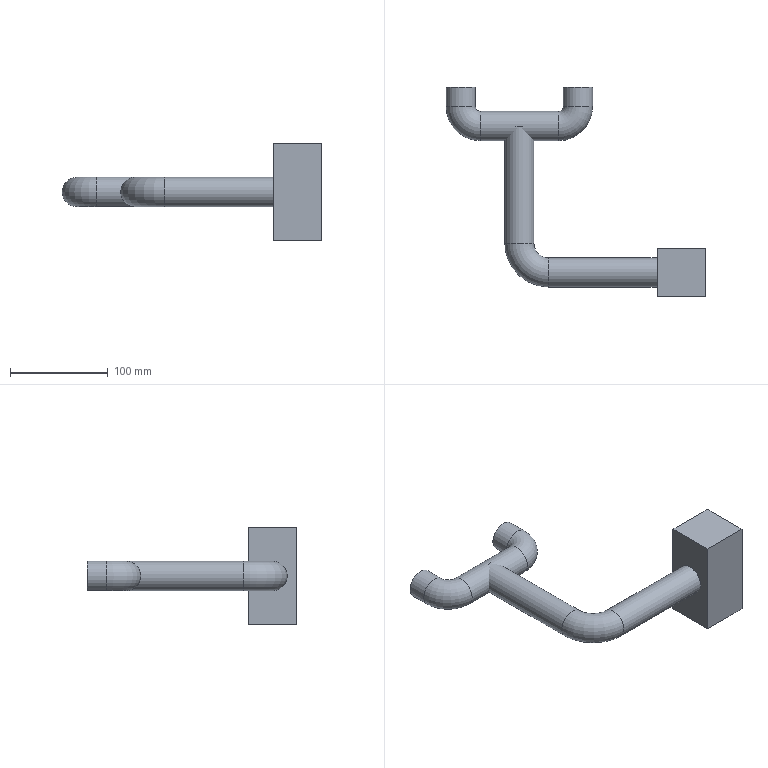Part | NX | features DATUM_CSYS 3, SKETCH 2, SWP104 2, EXTRUDE 1 | 2 solids | 17 faces | box 266 x 215 x 100 mm | volume 575830 mm3 | plane 9 | cylinder 5 | torus 3 | commonest cylinder face diameters 30 x5
STEP:
#1=CARTESIAN_POINT('',(-75.,20.,0.));
#2=VERTEX_POINT('',#1);
#3=CARTESIAN_POINT('',(-60.,20.,0.));
#4=DIRECTION('',(0.,1.,0.));
#5=DIRECTION('',(-1.,0.,0.));
#6=AXIS2_PLACEMENT_3D('',#3,#4,#5);
#7=CIRCLE('',#6,15.);
#8=EDGE_CURVE('',#2,#2,#7,.T.);
#9=ORIENTED_EDGE('',*,*,#8,.T.);
#10=EDGE_LOOP('',(#9));
#11=FACE_BOUND('',#10,.T.);
#12=CARTESIAN_POINT('',(-75.,40.,0.));
#13=VERTEX_POINT('',#12);
#14=CARTESIAN_POINT('',(-60.,40.,0.));
#15=DIRECTION('',(0.,1.,0.));
#16=DIRECTION('',(-1.,0.,0.));
#17=AXIS2_PLACEMENT_3D('',#14,#15,#16);
#18=CIRCLE('',#17,15.);
#19=EDGE_CURVE('',#13,#13,#18,.T.);
#20=ORIENTED_EDGE('',*,*,#19,.F.);
#21=EDGE_LOOP('',(#20));
#22=FACE_BOUND('',#21,.T.);
#23=CARTESIAN_POINT('',(-60.,20.,0.));
#24=DIRECTION('',(0.,1.,0.));
#25=DIRECTION('',(-1.,0.,0.));
#26=AXIS2_PLACEMENT_3D('',#23,#24,#25);
#27=CYLINDRICAL_SURFACE('',#26,15.);
#28=ADVANCED_FACE('',(#11,#22),#27,.T.);
#29=CARTESIAN_POINT('',(-40.,-15.,0.));
#30=VERTEX_POINT('',#29);
#31=CARTESIAN_POINT('',(-40.,0.,0.));
#32=DIRECTION('',(-1.,0.,0.));
#33=DIRECTION('',(0.,-1.,0.));
#34=AXIS2_PLACEMENT_3D('',#31,#32,#33);
#35=CIRCLE('',#34,15.);
#36=EDGE_CURVE('',#30,#30,#35,.T.);
#37=ORIENTED_EDGE('',*,*,#36,.T.);
#38=EDGE_LOOP('',(#37));
#39=FACE_BOUND('',#38,.T.);
#40=ORIENTED_EDGE('',*,*,#8,.F.);
#41=EDGE_LOOP('',(#40));
#42=FACE_BOUND('',#41,.T.);
#43=CARTESIAN_POINT('',(-40.,20.,0.));
#44=DIRECTION('',(0.,0.,-1.));
#45=DIRECTION('',(-1.,0.,0.));
#46=AXIS2_PLACEMENT_3D('',#43,#44,#45);
#47=TOROIDAL_SURFACE('',#46,20.,15.);
#48=ADVANCED_FACE('',(#39,#42),#47,.T.);
#49=CARTESIAN_POINT('',(40.,-15.,0.));
#50=VERTEX_POINT('',#49);
#51=CARTESIAN_POINT('',(40.,0.,0.));
#52=DIRECTION('',(-1.,0.,0.));
#53=DIRECTION('',(0.,-1.,0.));
#54=AXIS2_PLACEMENT_3D('',#51,#52,#53);
#55=CIRCLE('',#54,15.);
#56=EDGE_CURVE('',#50,#50,#55,.T.);
#57=ORIENTED_EDGE('',*,*,#56,.T.);
#58=EDGE_LOOP('',(#57));
#59=FACE_BOUND('',#58,.T.);
#60=ORIENTED_EDGE('',*,*,#36,.F.);
#61=EDGE_LOOP('',(#60));
#62=FACE_BOUND('',#61,.T.);
#63=CARTESIAN_POINT('',(40.,0.,0.));
#64=DIRECTION('',(-1.,0.,0.));
#65=DIRECTION('',(0.,0.,1.));
#66=AXIS2_PLACEMENT_3D('',#63,#64,#65);
#67=CYLINDRICAL_SURFACE('',#66,15.);
#68=ADVANCED_FACE('',(#59,#62),#67,.T.);
#69=CARTESIAN_POINT('',(75.,20.,0.));
#70=VERTEX_POINT('',#69);
#71=CARTESIAN_POINT('',(60.,20.,0.));
#72=DIRECTION('',(0.,-1.,0.));
#73=DIRECTION('',(1.,0.,0.));
#74=AXIS2_PLACEMENT_3D('',#71,#72,#73);
#75=CIRCLE('',#74,15.);
#76=EDGE_CURVE('',#70,#70,#75,.T.);
#77=ORIENTED_EDGE('',*,*,#76,.T.);
#78=EDGE_LOOP('',(#77));
#79=FACE_BOUND('',#78,.T.);
#80=ORIENTED_EDGE('',*,*,#56,.F.);
#81=EDGE_LOOP('',(#80));
#82=FACE_BOUND('',#81,.T.);
#83=CARTESIAN_POINT('',(40.,20.,0.));
#84=DIRECTION('',(0.,0.,-1.));
#85=DIRECTION('',(-1.,0.,0.));
#86=AXIS2_PLACEMENT_3D('',#83,#84,#85);
#87=TOROIDAL_SURFACE('',#86,20.,15.);
#88=ADVANCED_FACE('',(#79,#82),#87,.T.);
#89=ORIENTED_EDGE('',*,*,#76,.F.);
#90=EDGE_LOOP('',(#89));
#91=FACE_BOUND('',#90,.T.);
#92=CARTESIAN_POINT('',(75.,40.,0.));
#93=VERTEX_POINT('',#92);
#94=CARTESIAN_POINT('',(60.,40.,0.));
#95=DIRECTION('',(0.,-1.,0.));
#96=DIRECTION('',(1.,0.,0.));
#97=AXIS2_PLACEMENT_3D('',#94,#95,#96);
#98=CIRCLE('',#97,15.);
#99=EDGE_CURVE('',#93,#93,#98,.T.);
#100=ORIENTED_EDGE('',*,*,#99,.T.);
#101=EDGE_LOOP('',(#100));
#102=FACE_BOUND('',#101,.T.);
#103=CARTESIAN_POINT('',(60.,20.,0.));
#104=DIRECTION('',(0.,1.,0.));
#105=DIRECTION('',(-1.,0.,0.));
#106=AXIS2_PLACEMENT_3D('',#103,#104,#105);
#107=CYLINDRICAL_SURFACE('',#106,15.);
#108=ADVANCED_FACE('',(#91,#102),#107,.T.);
#109=ORIENTED_EDGE('',*,*,#19,.T.);
#110=EDGE_LOOP('',(#109));
#111=FACE_BOUND('',#110,.T.);
#112=CARTESIAN_POINT('',(-60.,40.,0.));
#113=DIRECTION('',(0.,1.,0.));
#114=DIRECTION('',(-1.,0.,0.));
#115=AXIS2_PLACEMENT_3D('',#112,#113,#114);
#116=PLANE('',#115);
#117=ADVANCED_FACE('',(#111),#116,.T.);
#118=ORIENTED_EDGE('',*,*,#99,.F.);
#119=EDGE_LOOP('',(#118));
#120=FACE_BOUND('',#119,.T.);
#121=CARTESIAN_POINT('',(60.,40.,0.));
#122=DIRECTION('',(0.,-1.,0.));
#123=DIRECTION('',(1.,0.,0.));
#124=AXIS2_PLACEMENT_3D('',#121,#122,#123);
#125=PLANE('',#124);
#126=ADVANCED_FACE('',(#120),#125,.F.);
#127=CLOSED_SHELL('',(#28,#48,#68,#88,#108,#117,#126));
#128=MANIFOLD_SOLID_BREP('',#127);
#129=CARTESIAN_POINT('',(0.,-120.,15.));
#130=VERTEX_POINT('',#129);
#131=CARTESIAN_POINT('',(0.,-120.,0.));
#132=DIRECTION('',(0.,1.,0.));
#133=DIRECTION('',(0.,0.,1.));
#134=AXIS2_PLACEMENT_3D('',#131,#132,#133);
#135=CIRCLE('',#134,15.);
#136=EDGE_CURVE('',#130,#130,#135,.T.);
#137=ORIENTED_EDGE('',*,*,#136,.T.);
#138=EDGE_LOOP('',(#137));
#139=FACE_BOUND('',#138,.T.);
#140=CARTESIAN_POINT('',(0.,0.,15.));
#141=VERTEX_POINT('',#140);
#142=CARTESIAN_POINT('',(0.,0.,0.));
#143=DIRECTION('',(0.,1.,0.));
#144=DIRECTION('',(0.,0.,1.));
#145=AXIS2_PLACEMENT_3D('',#142,#143,#144);
#146=CIRCLE('',#145,15.);
#147=EDGE_CURVE('',#141,#141,#146,.T.);
#148=ORIENTED_EDGE('',*,*,#147,.F.);
#149=EDGE_LOOP('',(#148));
#150=FACE_BOUND('',#149,.T.);
#151=CARTESIAN_POINT('',(0.,-120.,0.));
#152=DIRECTION('',(0.,1.,0.));
#153=DIRECTION('',(-1.,0.,0.));
#154=AXIS2_PLACEMENT_3D('',#151,#152,#153);
#155=CYLINDRICAL_SURFACE('',#154,15.);
#156=ADVANCED_FACE('',(#139,#150),#155,.T.);
#157=CARTESIAN_POINT('',(30.,-150.,15.));
#158=VERTEX_POINT('',#157);
#159=CARTESIAN_POINT('',(30.,-150.,0.));
#160=DIRECTION('',(-1.,0.,0.));
#161=DIRECTION('',(0.,0.,1.));
#162=AXIS2_PLACEMENT_3D('',#159,#160,#161);
#163=CIRCLE('',#162,15.);
#164=EDGE_CURVE('',#158,#158,#163,.T.);
#165=ORIENTED_EDGE('',*,*,#164,.T.);
#166=EDGE_LOOP('',(#165));
#167=FACE_BOUND('',#166,.T.);
#168=ORIENTED_EDGE('',*,*,#136,.F.);
#169=EDGE_LOOP('',(#168));
#170=FACE_BOUND('',#169,.T.);
#171=CARTESIAN_POINT('',(30.,-120.,0.));
#172=DIRECTION('',(0.,0.,-1.));
#173=DIRECTION('',(-1.,0.,0.));
#174=AXIS2_PLACEMENT_3D('',#171,#172,#173);
#175=TOROIDAL_SURFACE('',#174,30.,15.);
#176=ADVANCED_FACE('',(#167,#170),#175,.T.);
#177=ORIENTED_EDGE('',*,*,#164,.F.);
#178=EDGE_LOOP('',(#177));
#179=FACE_BOUND('',#178,.T.);
#180=CARTESIAN_POINT('',(141.,-150.,15.));
#181=VERTEX_POINT('',#180);
#182=CARTESIAN_POINT('',(141.,-150.,0.));
#183=DIRECTION('',(-1.,0.,0.));
#184=DIRECTION('',(0.,0.,1.));
#185=AXIS2_PLACEMENT_3D('',#182,#183,#184);
#186=CIRCLE('',#185,15.);
#187=EDGE_CURVE('',#181,#181,#186,.T.);
#188=ORIENTED_EDGE('',*,*,#187,.T.);
#189=EDGE_LOOP('',(#188));
#190=FACE_BOUND('',#189,.T.);
#191=CARTESIAN_POINT('',(30.,-150.,0.));
#192=DIRECTION('',(1.,0.,0.));
#193=DIRECTION('',(0.,0.,-1.));
#194=AXIS2_PLACEMENT_3D('',#191,#192,#193);
#195=CYLINDRICAL_SURFACE('',#194,15.);
#196=ADVANCED_FACE('',(#179,#190),#195,.T.);
#197=ORIENTED_EDGE('',*,*,#147,.T.);
#198=EDGE_LOOP('',(#197));
#199=FACE_BOUND('',#198,.T.);
#200=CARTESIAN_POINT('',(0.,0.,0.));
#201=DIRECTION('',(0.,1.,0.));
#202=DIRECTION('',(0.,0.,1.));
#203=AXIS2_PLACEMENT_3D('',#200,#201,#202);
#204=PLANE('',#203);
#205=ADVANCED_FACE('',(#199),#204,.T.);
#206=CARTESIAN_POINT('',(141.,-175.,-50.));
#207=VERTEX_POINT('',#206);
#208=CARTESIAN_POINT('',(191.,-175.,-50.));
#209=VERTEX_POINT('',#208);
#210=CARTESIAN_POINT('',(141.,-175.,-50.));
#211=DIRECTION('',(1.,0.,0.));
#212=VECTOR('',#211,1000.);
#213=LINE('',#210,#212);
#214=EDGE_CURVE('',#207,#209,#213,.T.);
#215=ORIENTED_EDGE('',*,*,#214,.T.);
#216=CARTESIAN_POINT('',(191.,-175.,50.));
#217=VERTEX_POINT('',#216);
#218=CARTESIAN_POINT('',(191.,-175.,50.));
#219=DIRECTION('',(0.,0.,-1.));
#220=VECTOR('',#219,1000.);
#221=LINE('',#218,#220);
#222=EDGE_CURVE('',#217,#209,#221,.T.);
#223=ORIENTED_EDGE('',*,*,#222,.F.);
#224=CARTESIAN_POINT('',(141.,-175.,50.));
#225=VERTEX_POINT('',#224);
#226=CARTESIAN_POINT('',(141.,-175.,50.));
#227=DIRECTION('',(1.,0.,0.));
#228=VECTOR('',#227,1000.);
#229=LINE('',#226,#228);
#230=EDGE_CURVE('',#225,#217,#229,.T.);
#231=ORIENTED_EDGE('',*,*,#230,.F.);
#232=CARTESIAN_POINT('',(141.,-175.,50.));
#233=DIRECTION('',(0.,0.,-1.));
#234=VECTOR('',#233,1000.);
#235=LINE('',#232,#234);
#236=EDGE_CURVE('',#225,#207,#235,.T.);
#237=ORIENTED_EDGE('',*,*,#236,.T.);
#238=EDGE_LOOP('',(#215,#223,#231,#237));
#239=FACE_BOUND('',#238,.T.);
#240=CARTESIAN_POINT('',(141.,-175.,50.));
#241=DIRECTION('',(0.,1.,0.));
#242=DIRECTION('',(0.,0.,1.));
#243=AXIS2_PLACEMENT_3D('',#240,#241,#242);
#244=PLANE('',#243);
#245=ADVANCED_FACE('',(#239),#244,.F.);
#246=CARTESIAN_POINT('',(191.,-125.,-50.));
#247=VERTEX_POINT('',#246);
#248=CARTESIAN_POINT('',(191.,-175.,-50.));
#249=DIRECTION('',(0.,1.,0.));
#250=VECTOR('',#249,1000.);
#251=LINE('',#248,#250);
#252=EDGE_CURVE('',#209,#247,#251,.T.);
#253=ORIENTED_EDGE('',*,*,#252,.T.);
#254=CARTESIAN_POINT('',(191.,-125.,50.));
#255=VERTEX_POINT('',#254);
#256=CARTESIAN_POINT('',(191.,-125.,50.));
#257=DIRECTION('',(0.,0.,-1.));
#258=VECTOR('',#257,1000.);
#259=LINE('',#256,#258);
#260=EDGE_CURVE('',#255,#247,#259,.T.);
#261=ORIENTED_EDGE('',*,*,#260,.F.);
#262=CARTESIAN_POINT('',(191.,-175.,50.));
#263=DIRECTION('',(0.,1.,0.));
#264=VECTOR('',#263,1000.);
#265=LINE('',#262,#264);
#266=EDGE_CURVE('',#217,#255,#265,.T.);
#267=ORIENTED_EDGE('',*,*,#266,.F.);
#268=ORIENTED_EDGE('',*,*,#222,.T.);
#269=EDGE_LOOP('',(#253,#261,#267,#268));
#270=FACE_BOUND('',#269,.T.);
#271=CARTESIAN_POINT('',(191.,-175.,50.));
#272=DIRECTION('',(-1.,0.,0.));
#273=DIRECTION('',(0.,0.,1.));
#274=AXIS2_PLACEMENT_3D('',#271,#272,#273);
#275=PLANE('',#274);
#276=ADVANCED_FACE('',(#270),#275,.F.);
#277=CARTESIAN_POINT('',(141.,-125.,-50.));
#278=VERTEX_POINT('',#277);
#279=CARTESIAN_POINT('',(191.,-125.,-50.));
#280=DIRECTION('',(-1.,0.,0.));
#281=VECTOR('',#280,1000.);
#282=LINE('',#279,#281);
#283=EDGE_CURVE('',#247,#278,#282,.T.);
#284=ORIENTED_EDGE('',*,*,#283,.T.);
#285=CARTESIAN_POINT('',(141.,-125.,50.));
#286=VERTEX_POINT('',#285);
#287=CARTESIAN_POINT('',(141.,-125.,50.));
#288=DIRECTION('',(0.,0.,-1.));
#289=VECTOR('',#288,1000.);
#290=LINE('',#287,#289);
#291=EDGE_CURVE('',#286,#278,#290,.T.);
#292=ORIENTED_EDGE('',*,*,#291,.F.);
#293=CARTESIAN_POINT('',(191.,-125.,50.));
#294=DIRECTION('',(-1.,0.,0.));
#295=VECTOR('',#294,1000.);
#296=LINE('',#293,#295);
#297=EDGE_CURVE('',#255,#286,#296,.T.);
#298=ORIENTED_EDGE('',*,*,#297,.F.);
#299=ORIENTED_EDGE('',*,*,#260,.T.);
#300=EDGE_LOOP('',(#284,#292,#298,#299));
#301=FACE_BOUND('',#300,.T.);
#302=CARTESIAN_POINT('',(191.,-125.,50.));
#303=DIRECTION('',(0.,-1.,0.));
#304=DIRECTION('',(1.,0.,0.));
#305=AXIS2_PLACEMENT_3D('',#302,#303,#304);
#306=PLANE('',#305);
#307=ADVANCED_FACE('',(#301),#306,.F.);
#308=ORIENTED_EDGE('',*,*,#187,.F.);
#309=EDGE_LOOP('',(#308));
#310=FACE_BOUND('',#309,.T.);
#311=CARTESIAN_POINT('',(141.,-125.,-50.));
#312=DIRECTION('',(0.,-1.,0.));
#313=VECTOR('',#312,1000.);
#314=LINE('',#311,#313);
#315=EDGE_CURVE('',#278,#207,#314,.T.);
#316=ORIENTED_EDGE('',*,*,#315,.T.);
#317=ORIENTED_EDGE('',*,*,#236,.F.);
#318=CARTESIAN_POINT('',(141.,-150.,50.));
#319=DIRECTION('',(0.,-1.,0.));
#320=VECTOR('',#319,1000.);
#321=LINE('',#318,#320);
#322=EDGE_CURVE('',#286,#225,#321,.T.);
#323=ORIENTED_EDGE('',*,*,#322,.F.);
#324=ORIENTED_EDGE('',*,*,#291,.T.);
#325=EDGE_LOOP('',(#316,#317,#323,#324));
#326=FACE_BOUND('',#325,.T.);
#327=CARTESIAN_POINT('',(141.,-125.,50.));
#328=DIRECTION('',(1.,0.,0.));
#329=DIRECTION('',(0.,0.,-1.));
#330=AXIS2_PLACEMENT_3D('',#327,#328,#329);
#331=PLANE('',#330);
#332=ADVANCED_FACE('',(#310,#326),#331,.F.);
#333=ORIENTED_EDGE('',*,*,#322,.T.);
#334=ORIENTED_EDGE('',*,*,#230,.T.);
#335=ORIENTED_EDGE('',*,*,#266,.T.);
#336=ORIENTED_EDGE('',*,*,#297,.T.);
#337=EDGE_LOOP('',(#333,#334,#335,#336));
#338=FACE_BOUND('',#337,.T.);
#339=CARTESIAN_POINT('',(0.,0.,50.));
#340=DIRECTION('',(0.,0.,1.));
#341=DIRECTION('',(1.,0.,0.));
#342=AXIS2_PLACEMENT_3D('',#339,#340,#341);
#343=PLANE('',#342);
#344=ADVANCED_FACE('',(#338),#343,.T.);
#345=ORIENTED_EDGE('',*,*,#214,.F.);
#346=ORIENTED_EDGE('',*,*,#315,.F.);
#347=ORIENTED_EDGE('',*,*,#283,.F.);
#348=ORIENTED_EDGE('',*,*,#252,.F.);
#349=EDGE_LOOP('',(#345,#346,#347,#348));
#350=FACE_BOUND('',#349,.T.);
#351=CARTESIAN_POINT('',(0.,0.,-50.));
#352=DIRECTION('',(0.,0.,1.));
#353=DIRECTION('',(1.,0.,0.));
#354=AXIS2_PLACEMENT_3D('',#351,#352,#353);
#355=PLANE('',#354);
#356=ADVANCED_FACE('',(#350),#355,.F.);
#357=CLOSED_SHELL('',(#156,#176,#196,#205,#245,#276,#307,#332,#344,#356));
#358=MANIFOLD_SOLID_BREP('',#357);
#359=(LENGTH_UNIT()NAMED_UNIT(*)SI_UNIT(.MILLI.,.METRE.));
#360=UNCERTAINTY_MEASURE_WITH_UNIT(LENGTH_MEASURE(0.00001),#359,'','');
#361=(NAMED_UNIT(*)PLANE_ANGLE_UNIT()SI_UNIT($,.RADIAN.));
#362=(NAMED_UNIT(*)SI_UNIT($,.STERADIAN.)SOLID_ANGLE_UNIT());
#363=(GEOMETRIC_REPRESENTATION_CONTEXT(3)GLOBAL_UNCERTAINTY_ASSIGNED_CONTEXT((#360))GLOBAL_UNIT_ASSIGNED_CONTEXT((#359,#361,#362))REPRESENTATION_CONTEXT('',''));
#364=ADVANCED_BREP_SHAPE_REPRESENTATION('',(#128,#358),#363);